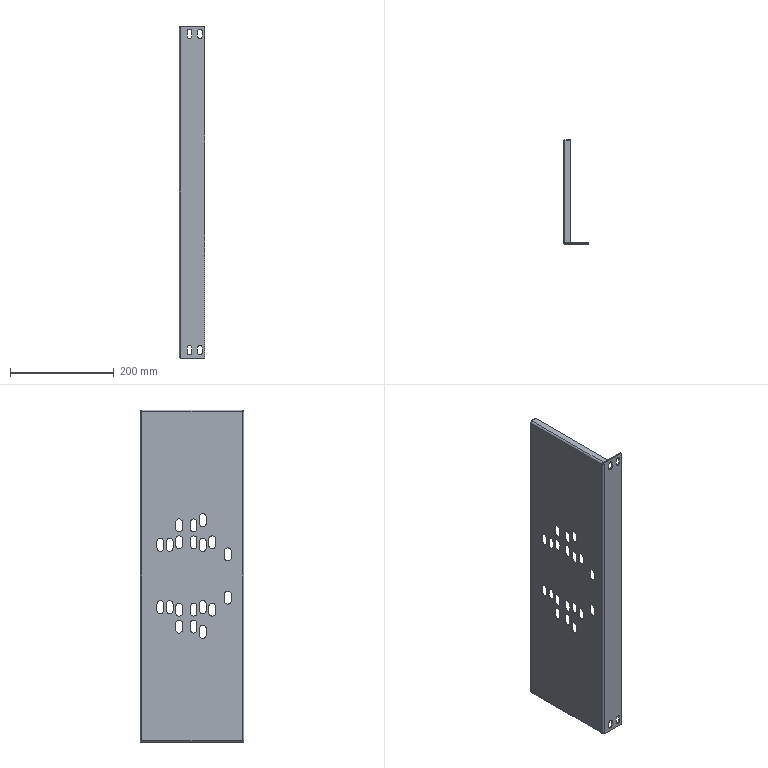Part | STEP file | Zero-sequence current transformer mounting plate | 1 solid | 142 faces | box 50 x 200 x 640 mm | volume 327853 mm3 | plane 86 | cylinder 56 | commonest cylinder face diameters 13 x40 9 x8 3 x4 7 x4